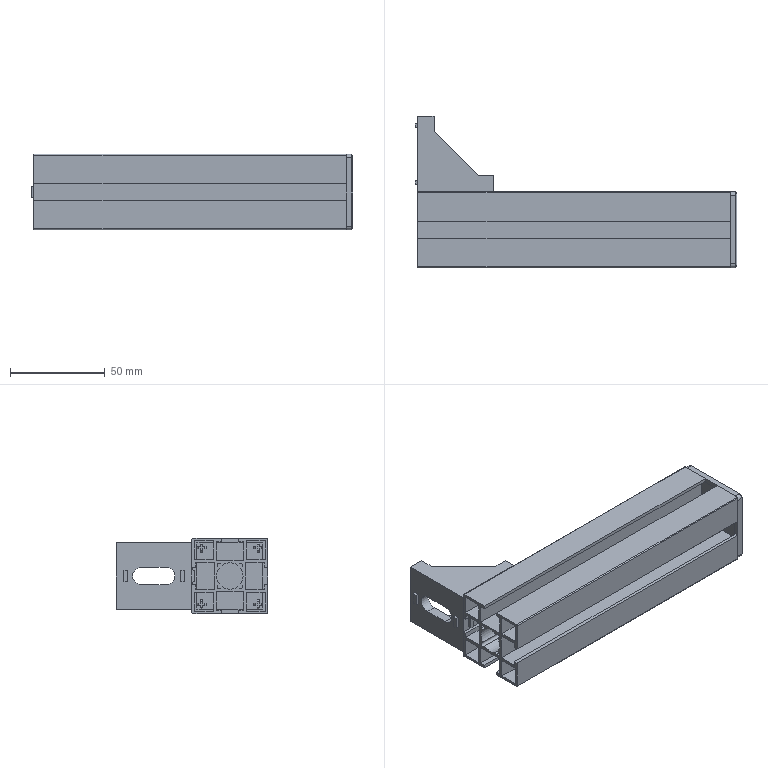Part | 3 solids | 244 faces | box 170 x 80 x 40 mm | volume 84807 mm3 | plane 181 | cylinder 39 | cone 24 | commonest cylinder face diameters 1.5 x16 2.2 x6 14 x5 1 x4 4 x4 9.2 x4